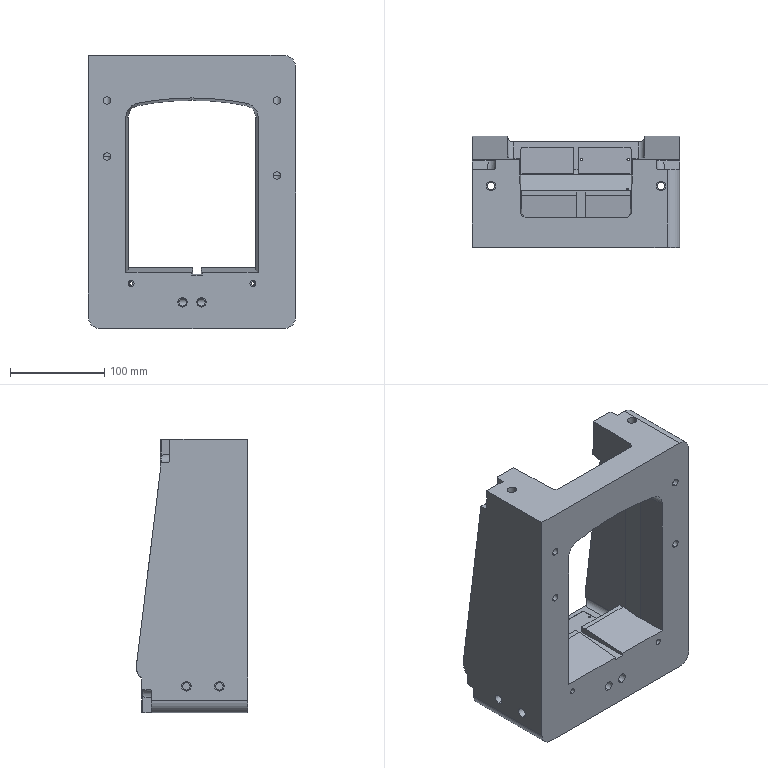Part | STEP file | 1 solid | 304 faces | box 220 x 118.069 x 290 mm | volume 3396178 mm3 | cylinder 133 | plane 91 | spline 48 | cone 14 | torus 14 | other 4 | commonest cylinder face diameters 8 x60 10 x24 2.513 x7 2.01 x5 3.5 x4 4.02 x4